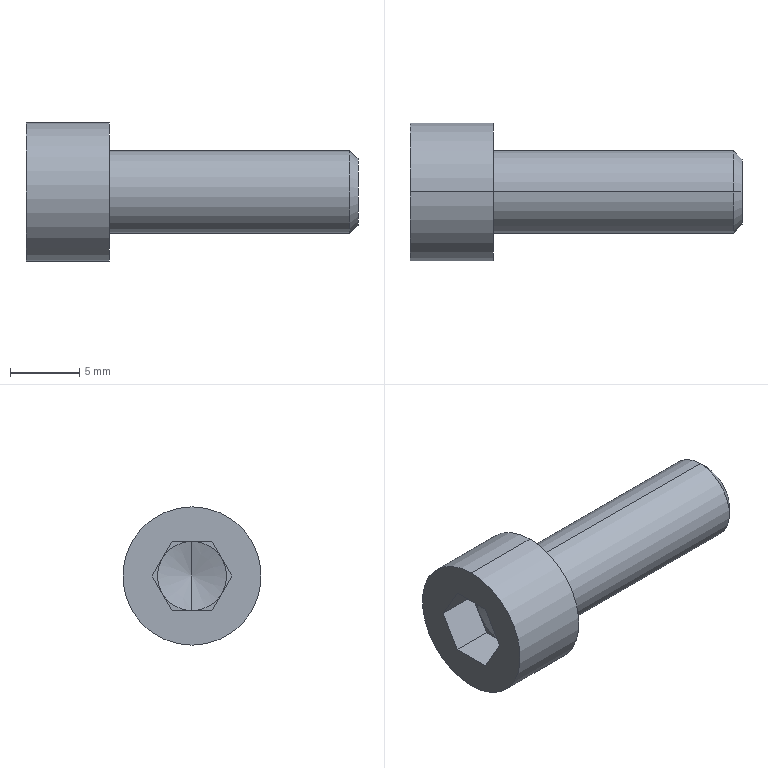Part | STEP file | CB6X1-L18-A10-E6-B5 | 1 solid | 23 faces | box 24 x 10 x 10 mm | volume 907.535 mm3 | plane 15 | cylinder 4 | cone 4 | commonest cylinder face diameters 6 x2 10 x2